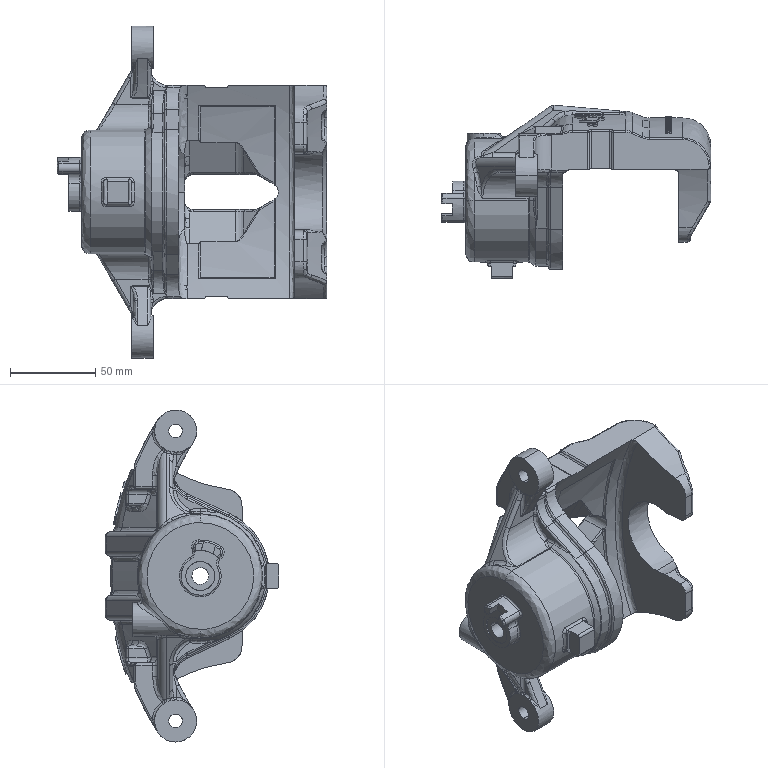Part | SolidWorks | features BaseBody 1 | 1 solid | 1195 faces | box 158.2 x 101.79 x 194.7 mm | volume 429554 mm3 | spline 696 | cylinder 241 | plane 228 | cone 30 | commonest cylinder face diameters 2 x42 6 x32 3 x23 4 x22 334.4 x16 10 x13